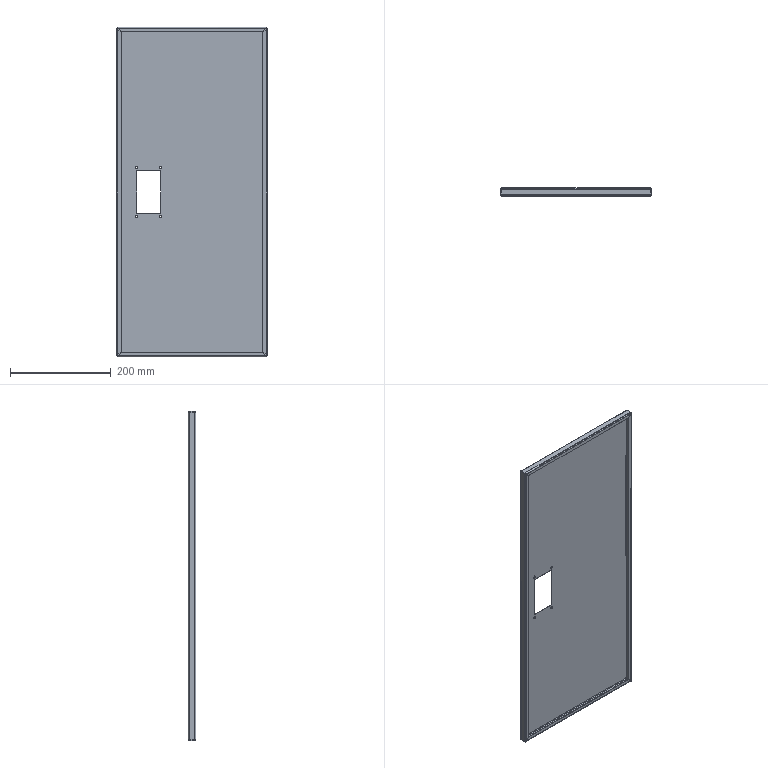Part | STEP file | 冲床-300配套压波_id342_x_t | 1 solid | 112 faces | box 300 x 15 x 655 mm | volume 275574 mm3 | spline 48 | plane 44 | cylinder 20 | commonest cylinder face diameters 3 x8 5.4 x8 4.5 x4